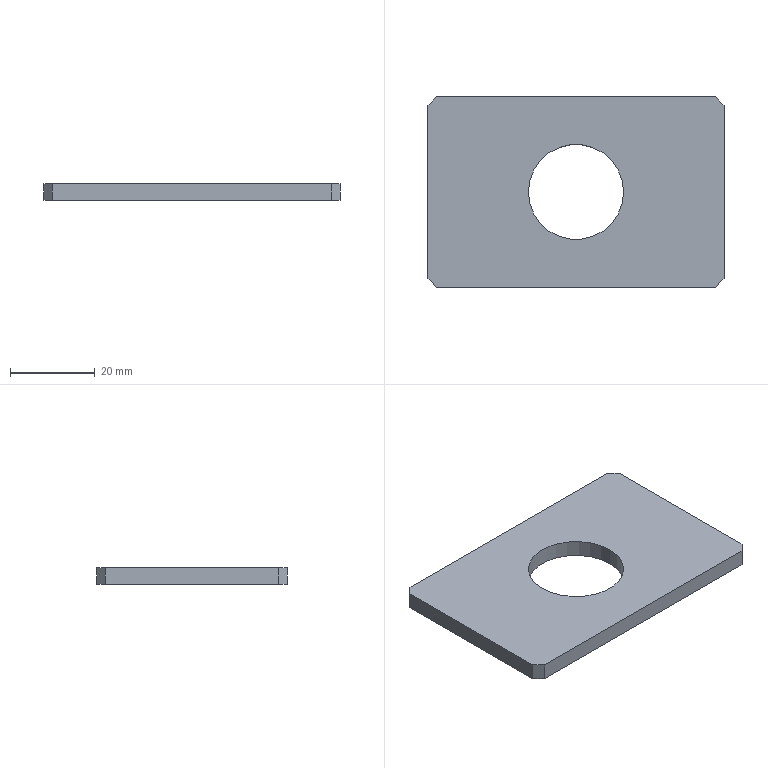Part | STEP file | Backup 2012-3-22-013 | 1 solid | 12 faces | box 70 x 45 x 4 mm | volume 10978 mm3 | plane 10 | cylinder 2 | commonest cylinder face diameters 22.5 x2
STEP:
#1=CARTESIAN_POINT('',(0.,0.,0.));
#2=DIRECTION('',(0.,0.,1.));
#3=DIRECTION('',(1.,0.,0.));
#4=AXIS2_PLACEMENT_3D('',#1,#2,#3);
#5=CARTESIAN_POINT('',(-11.25,0.,4.));
#6=VERTEX_POINT('',#5);
#7=CARTESIAN_POINT('',(-11.25,0.,0.));
#8=VERTEX_POINT('',#7);
#9=CARTESIAN_POINT('',(-11.25,0.,4.));
#10=DIRECTION('',(0.,0.,-1.));
#11=VECTOR('',#10,1.);
#12=LINE('',#9,#11);
#13=CARTESIAN_POINT('',(0.,0.,4.));
#14=DIRECTION('',(0.,0.,-1.));
#15=DIRECTION('',(-1.,0.,0.));
#16=AXIS2_PLACEMENT_3D('',#13,#14,#15);
#17=CYLINDRICAL_SURFACE('',#16,11.25);
#18=CARTESIAN_POINT('',(6.283,0.));
#19=DIRECTION('',(0.,1.));
#20=VECTOR('',#19,1.);
#21=LINE('',#18,#20);
#22=(GEOMETRIC_REPRESENTATION_CONTEXT(2)PARAMETRIC_REPRESENTATION_CONTEXT()REPRESENTATION_CONTEXT('',''));
#23=DEFINITIONAL_REPRESENTATION('',(#21),#22);
#24=PCURVE('',#17,#23);
#25=CARTESIAN_POINT('',(0.,0.,4.));
#26=DIRECTION('',(0.,0.,-1.));
#27=DIRECTION('',(-1.,0.,0.));
#28=AXIS2_PLACEMENT_3D('',#25,#26,#27);
#29=CYLINDRICAL_SURFACE('',#28,11.25);
#30=CARTESIAN_POINT('',(0.,0.));
#31=DIRECTION('',(0.,1.));
#32=VECTOR('',#31,1.);
#33=LINE('',#30,#32);
#34=(GEOMETRIC_REPRESENTATION_CONTEXT(2)PARAMETRIC_REPRESENTATION_CONTEXT()REPRESENTATION_CONTEXT('',''));
#35=DEFINITIONAL_REPRESENTATION('',(#33),#34);
#36=PCURVE('',#29,#35);
#37=SURFACE_CURVE('',#12,(#24,#36),.PCURVE_S1.);
#38=EDGE_CURVE('',#6,#8,#37,.T.);
#39=ORIENTED_EDGE('',*,*,#38,.T.);
#40=CARTESIAN_POINT('',(11.25,0.,0.));
#41=VERTEX_POINT('',#40);
#42=CARTESIAN_POINT('',(0.,0.,0.));
#43=DIRECTION('',(0.,0.,1.));
#44=DIRECTION('',(1.,0.,0.));
#45=AXIS2_PLACEMENT_3D('',#42,#43,#44);
#46=CIRCLE('',#45,11.25);
#47=CARTESIAN_POINT('',(9.425,4.));
#48=DIRECTION('',(-1.,0.));
#49=VECTOR('',#48,1.);
#50=LINE('',#47,#49);
#51=(GEOMETRIC_REPRESENTATION_CONTEXT(2)PARAMETRIC_REPRESENTATION_CONTEXT()REPRESENTATION_CONTEXT('',''));
#52=DEFINITIONAL_REPRESENTATION('',(#50),#51);
#53=PCURVE('',#17,#52);
#54=CARTESIAN_POINT('',(35.,-22.5,0.));
#55=DIRECTION('',(0.,0.,1.));
#56=DIRECTION('',(1.,0.,0.));
#57=AXIS2_PLACEMENT_3D('',#54,#55,#56);
#58=PLANE('',#57);
#59=CARTESIAN_POINT('',(-35.,22.5));
#60=DIRECTION('',(1.,0.));
#61=AXIS2_PLACEMENT_2D('',#59,#60);
#62=CIRCLE('',#61,11.25);
#63=(GEOMETRIC_REPRESENTATION_CONTEXT(2)PARAMETRIC_REPRESENTATION_CONTEXT()REPRESENTATION_CONTEXT('',''));
#64=DEFINITIONAL_REPRESENTATION('',(#62),#63);
#65=PCURVE('',#58,#64);
#66=SURFACE_CURVE('',#46,(#53,#65),.PCURVE_S1.);
#67=EDGE_CURVE('',#8,#41,#66,.T.);
#68=ORIENTED_EDGE('',*,*,#67,.T.);
#69=CARTESIAN_POINT('',(11.25,0.,4.));
#70=VERTEX_POINT('',#69);
#71=CARTESIAN_POINT('',(11.25,0.,4.));
#72=DIRECTION('',(0.,0.,-1.));
#73=VECTOR('',#72,1.);
#74=LINE('',#71,#73);
#75=CARTESIAN_POINT('',(3.142,0.));
#76=DIRECTION('',(0.,1.));
#77=VECTOR('',#76,1.);
#78=LINE('',#75,#77);
#79=(GEOMETRIC_REPRESENTATION_CONTEXT(2)PARAMETRIC_REPRESENTATION_CONTEXT()REPRESENTATION_CONTEXT('',''));
#80=DEFINITIONAL_REPRESENTATION('',(#78),#79);
#81=PCURVE('',#17,#80);
#82=CARTESIAN_POINT('',(3.142,0.));
#83=DIRECTION('',(0.,1.));
#84=VECTOR('',#83,1.);
#85=LINE('',#82,#84);
#86=(GEOMETRIC_REPRESENTATION_CONTEXT(2)PARAMETRIC_REPRESENTATION_CONTEXT()REPRESENTATION_CONTEXT('',''));
#87=DEFINITIONAL_REPRESENTATION('',(#85),#86);
#88=PCURVE('',#29,#87);
#89=SURFACE_CURVE('',#74,(#81,#88),.PCURVE_S1.);
#90=EDGE_CURVE('',#70,#41,#89,.T.);
#91=ORIENTED_EDGE('',*,*,#90,.F.);
#92=CARTESIAN_POINT('',(0.,0.,4.));
#93=DIRECTION('',(0.,0.,1.));
#94=DIRECTION('',(1.,0.,0.));
#95=AXIS2_PLACEMENT_3D('',#92,#93,#94);
#96=CIRCLE('',#95,11.25);
#97=CARTESIAN_POINT('',(9.425,0.));
#98=DIRECTION('',(-1.,0.));
#99=VECTOR('',#98,1.);
#100=LINE('',#97,#99);
#101=(GEOMETRIC_REPRESENTATION_CONTEXT(2)PARAMETRIC_REPRESENTATION_CONTEXT()REPRESENTATION_CONTEXT('',''));
#102=DEFINITIONAL_REPRESENTATION('',(#100),#101);
#103=PCURVE('',#17,#102);
#104=CARTESIAN_POINT('',(35.,-22.5,4.));
#105=DIRECTION('',(0.,0.,1.));
#106=DIRECTION('',(1.,0.,0.));
#107=AXIS2_PLACEMENT_3D('',#104,#105,#106);
#108=PLANE('',#107);
#109=CARTESIAN_POINT('',(-35.,22.5));
#110=DIRECTION('',(1.,0.));
#111=AXIS2_PLACEMENT_2D('',#109,#110);
#112=CIRCLE('',#111,11.25);
#113=(GEOMETRIC_REPRESENTATION_CONTEXT(2)PARAMETRIC_REPRESENTATION_CONTEXT()REPRESENTATION_CONTEXT('',''));
#114=DEFINITIONAL_REPRESENTATION('',(#112),#113);
#115=PCURVE('',#108,#114);
#116=SURFACE_CURVE('',#96,(#103,#115),.PCURVE_S1.);
#117=EDGE_CURVE('',#6,#70,#116,.T.);
#118=ORIENTED_EDGE('',*,*,#117,.F.);
#119=EDGE_LOOP('',(#39,#68,#91,#118));
#120=FACE_BOUND('',#119,.F.);
#121=ADVANCED_FACE('',(#120),#17,.F.);
#122=CARTESIAN_POINT('',(-35.,20.5,4.));
#123=VERTEX_POINT('',#122);
#124=CARTESIAN_POINT('',(-35.,-20.5,4.));
#125=VERTEX_POINT('',#124);
#126=CARTESIAN_POINT('',(-35.,22.5,4.));
#127=DIRECTION('',(0.,-1.,0.));
#128=VECTOR('',#127,1.);
#129=LINE('',#126,#128);
#130=CARTESIAN_POINT('',(-70.,45.));
#131=DIRECTION('',(0.,-1.));
#132=VECTOR('',#131,1.);
#133=LINE('',#130,#132);
#134=(GEOMETRIC_REPRESENTATION_CONTEXT(2)PARAMETRIC_REPRESENTATION_CONTEXT()REPRESENTATION_CONTEXT('',''));
#135=DEFINITIONAL_REPRESENTATION('',(#133),#134);
#136=PCURVE('',#108,#135);
#137=CARTESIAN_POINT('',(-35.,22.5,4.));
#138=DIRECTION('',(1.,0.,0.));
#139=DIRECTION('',(0.,1.,0.));
#140=AXIS2_PLACEMENT_3D('',#137,#138,#139);
#141=PLANE('',#140);
#142=CARTESIAN_POINT('',(0.,0.));
#143=DIRECTION('',(-1.,0.));
#144=VECTOR('',#143,1.);
#145=LINE('',#142,#144);
#146=(GEOMETRIC_REPRESENTATION_CONTEXT(2)PARAMETRIC_REPRESENTATION_CONTEXT()REPRESENTATION_CONTEXT('',''));
#147=DEFINITIONAL_REPRESENTATION('',(#145),#146);
#148=PCURVE('',#141,#147);
#149=SURFACE_CURVE('',#129,(#136,#148),.PCURVE_S1.);
#150=EDGE_CURVE('',#123,#125,#149,.T.);
#151=ORIENTED_EDGE('',*,*,#150,.T.);
#152=CARTESIAN_POINT('',(-33.,-22.5,4.));
#153=VERTEX_POINT('',#152);
#154=CARTESIAN_POINT('',(1.,-56.5,4.));
#155=DIRECTION('',(0.7071,-0.7071,0.));
#156=VECTOR('',#155,1.);
#157=LINE('',#154,#156);
#158=CARTESIAN_POINT('',(-34.,-34.));
#159=DIRECTION('',(0.7071,-0.7071));
#160=VECTOR('',#159,1.);
#161=LINE('',#158,#160);
#162=(GEOMETRIC_REPRESENTATION_CONTEXT(2)PARAMETRIC_REPRESENTATION_CONTEXT()REPRESENTATION_CONTEXT('',''));
#163=DEFINITIONAL_REPRESENTATION('',(#161),#162);
#164=PCURVE('',#108,#163);
#165=CARTESIAN_POINT('',(-33.,-22.5,4.));
#166=DIRECTION('',(0.7071,0.7071,0.));
#167=DIRECTION('',(-0.7071,0.7071,0.));
#168=AXIS2_PLACEMENT_3D('',#165,#166,#167);
#169=PLANE('',#168);
#170=CARTESIAN_POINT('',(-48.083,0.));
#171=DIRECTION('',(-1.,0.));
#172=VECTOR('',#171,1.);
#173=LINE('',#170,#172);
#174=(GEOMETRIC_REPRESENTATION_CONTEXT(2)PARAMETRIC_REPRESENTATION_CONTEXT()REPRESENTATION_CONTEXT('',''));
#175=DEFINITIONAL_REPRESENTATION('',(#173),#174);
#176=PCURVE('',#169,#175);
#177=SURFACE_CURVE('',#157,(#164,#176),.PCURVE_S1.);
#178=EDGE_CURVE('',#125,#153,#177,.T.);
#179=ORIENTED_EDGE('',*,*,#178,.T.);
#180=CARTESIAN_POINT('',(33.,-22.5,4.));
#181=VERTEX_POINT('',#180);
#182=CARTESIAN_POINT('',(-35.,-22.5,4.));
#183=DIRECTION('',(1.,0.,0.));
#184=VECTOR('',#183,1.);
#185=LINE('',#182,#184);
#186=CARTESIAN_POINT('',(-70.,0.));
#187=DIRECTION('',(1.,0.));
#188=VECTOR('',#187,1.);
#189=LINE('',#186,#188);
#190=(GEOMETRIC_REPRESENTATION_CONTEXT(2)PARAMETRIC_REPRESENTATION_CONTEXT()REPRESENTATION_CONTEXT('',''));
#191=DEFINITIONAL_REPRESENTATION('',(#189),#190);
#192=PCURVE('',#108,#191);
#193=CARTESIAN_POINT('',(-35.,-22.5,4.));
#194=DIRECTION('',(0.,1.,0.));
#195=DIRECTION('',(0.,0.,1.));
#196=AXIS2_PLACEMENT_3D('',#193,#194,#195);
#197=PLANE('',#196);
#198=CARTESIAN_POINT('',(0.,0.));
#199=DIRECTION('',(0.,1.));
#200=VECTOR('',#199,1.);
#201=LINE('',#198,#200);
#202=(GEOMETRIC_REPRESENTATION_CONTEXT(2)PARAMETRIC_REPRESENTATION_CONTEXT()REPRESENTATION_CONTEXT('',''));
#203=DEFINITIONAL_REPRESENTATION('',(#201),#202);
#204=PCURVE('',#197,#203);
#205=SURFACE_CURVE('',#185,(#192,#204),.PCURVE_S1.);
#206=EDGE_CURVE('',#153,#181,#205,.T.);
#207=ORIENTED_EDGE('',*,*,#206,.T.);
#208=CARTESIAN_POINT('',(35.,-20.5,4.));
#209=VERTEX_POINT('',#208);
#210=CARTESIAN_POINT('',(34.,-21.5,4.));
#211=DIRECTION('',(0.7071,0.7071,0.));
#212=VECTOR('',#211,1.);
#213=LINE('',#210,#212);
#214=CARTESIAN_POINT('',(-1.,1.));
#215=DIRECTION('',(0.7071,0.7071));
#216=VECTOR('',#215,1.);
#217=LINE('',#214,#216);
#218=(GEOMETRIC_REPRESENTATION_CONTEXT(2)PARAMETRIC_REPRESENTATION_CONTEXT()REPRESENTATION_CONTEXT('',''));
#219=DEFINITIONAL_REPRESENTATION('',(#217),#218);
#220=PCURVE('',#108,#219);
#221=CARTESIAN_POINT('',(35.,-20.5,4.));
#222=DIRECTION('',(-0.7071,0.7071,0.));
#223=DIRECTION('',(-0.7071,-0.7071,0.));
#224=AXIS2_PLACEMENT_3D('',#221,#222,#223);
#225=PLANE('',#224);
#226=CARTESIAN_POINT('',(1.414,0.));
#227=DIRECTION('',(-1.,0.));
#228=VECTOR('',#227,1.);
#229=LINE('',#226,#228);
#230=(GEOMETRIC_REPRESENTATION_CONTEXT(2)PARAMETRIC_REPRESENTATION_CONTEXT()REPRESENTATION_CONTEXT('',''));
#231=DEFINITIONAL_REPRESENTATION('',(#229),#230);
#232=PCURVE('',#225,#231);
#233=SURFACE_CURVE('',#213,(#220,#232),.PCURVE_S1.);
#234=EDGE_CURVE('',#181,#209,#233,.T.);
#235=ORIENTED_EDGE('',*,*,#234,.T.);
#236=CARTESIAN_POINT('',(35.,20.5,4.));
#237=VERTEX_POINT('',#236);
#238=CARTESIAN_POINT('',(35.,22.5,4.));
#239=DIRECTION('',(0.,1.,0.));
#240=VECTOR('',#239,1.);
#241=LINE('',#238,#240);
#242=CARTESIAN_POINT('',(0.,45.));
#243=DIRECTION('',(0.,1.));
#244=VECTOR('',#243,1.);
#245=LINE('',#242,#244);
#246=(GEOMETRIC_REPRESENTATION_CONTEXT(2)PARAMETRIC_REPRESENTATION_CONTEXT()REPRESENTATION_CONTEXT('',''));
#247=DEFINITIONAL_REPRESENTATION('',(#245),#246);
#248=PCURVE('',#108,#247);
#249=CARTESIAN_POINT('',(35.,22.5,4.));
#250=DIRECTION('',(-1.,0.,0.));
#251=DIRECTION('',(0.,-1.,0.));
#252=AXIS2_PLACEMENT_3D('',#249,#250,#251);
#253=PLANE('',#252);
#254=CARTESIAN_POINT('',(0.,0.));
#255=DIRECTION('',(-1.,0.));
#256=VECTOR('',#255,1.);
#257=LINE('',#254,#256);
#258=(GEOMETRIC_REPRESENTATION_CONTEXT(2)PARAMETRIC_REPRESENTATION_CONTEXT()REPRESENTATION_CONTEXT('',''));
#259=DEFINITIONAL_REPRESENTATION('',(#257),#258);
#260=PCURVE('',#253,#259);
#261=SURFACE_CURVE('',#241,(#248,#260),.PCURVE_S1.);
#262=EDGE_CURVE('',#209,#237,#261,.T.);
#263=ORIENTED_EDGE('',*,*,#262,.T.);
#264=CARTESIAN_POINT('',(33.,22.5,4.));
#265=VERTEX_POINT('',#264);
#266=CARTESIAN_POINT('',(56.5,-1.,4.));
#267=DIRECTION('',(-0.7071,0.7071,0.));
#268=VECTOR('',#267,1.);
#269=LINE('',#266,#268);
#270=CARTESIAN_POINT('',(21.5,21.5));
#271=DIRECTION('',(-0.7071,0.7071));
#272=VECTOR('',#271,1.);
#273=LINE('',#270,#272);
#274=(GEOMETRIC_REPRESENTATION_CONTEXT(2)PARAMETRIC_REPRESENTATION_CONTEXT()REPRESENTATION_CONTEXT('',''));
#275=DEFINITIONAL_REPRESENTATION('',(#273),#274);
#276=PCURVE('',#108,#275);
#277=CARTESIAN_POINT('',(33.,22.5,4.));
#278=DIRECTION('',(-0.7071,-0.7071,0.));
#279=DIRECTION('',(0.7071,-0.7071,0.));
#280=AXIS2_PLACEMENT_3D('',#277,#278,#279);
#281=PLANE('',#280);
#282=CARTESIAN_POINT('',(33.234,0.));
#283=DIRECTION('',(-1.,0.));
#284=VECTOR('',#283,1.);
#285=LINE('',#282,#284);
#286=(GEOMETRIC_REPRESENTATION_CONTEXT(2)PARAMETRIC_REPRESENTATION_CONTEXT()REPRESENTATION_CONTEXT('',''));
#287=DEFINITIONAL_REPRESENTATION('',(#285),#286);
#288=PCURVE('',#281,#287);
#289=SURFACE_CURVE('',#269,(#276,#288),.PCURVE_S1.);
#290=EDGE_CURVE('',#237,#265,#289,.T.);
#291=ORIENTED_EDGE('',*,*,#290,.T.);
#292=CARTESIAN_POINT('',(-33.,22.5,4.));
#293=VERTEX_POINT('',#292);
#294=CARTESIAN_POINT('',(-35.,22.5,4.));
#295=DIRECTION('',(-1.,0.,0.));
#296=VECTOR('',#295,1.);
#297=LINE('',#294,#296);
#298=CARTESIAN_POINT('',(-70.,45.));
#299=DIRECTION('',(-1.,0.));
#300=VECTOR('',#299,1.);
#301=LINE('',#298,#300);
#302=(GEOMETRIC_REPRESENTATION_CONTEXT(2)PARAMETRIC_REPRESENTATION_CONTEXT()REPRESENTATION_CONTEXT('',''));
#303=DEFINITIONAL_REPRESENTATION('',(#301),#302);
#304=PCURVE('',#108,#303);
#305=CARTESIAN_POINT('',(-35.,22.5,4.));
#306=DIRECTION('',(0.,-1.,0.));
#307=DIRECTION('',(0.,0.,-1.));
#308=AXIS2_PLACEMENT_3D('',#305,#306,#307);
#309=PLANE('',#308);
#310=CARTESIAN_POINT('',(0.,0.));
#311=DIRECTION('',(0.,-1.));
#312=VECTOR('',#311,1.);
#313=LINE('',#310,#312);
#314=(GEOMETRIC_REPRESENTATION_CONTEXT(2)PARAMETRIC_REPRESENTATION_CONTEXT()REPRESENTATION_CONTEXT('',''));
#315=DEFINITIONAL_REPRESENTATION('',(#313),#314);
#316=PCURVE('',#309,#315);
#317=SURFACE_CURVE('',#297,(#304,#316),.PCURVE_S1.);
#318=EDGE_CURVE('',#265,#293,#317,.T.);
#319=ORIENTED_EDGE('',*,*,#318,.T.);
#320=CARTESIAN_POINT('',(-21.5,34.,4.));
#321=DIRECTION('',(-0.7071,-0.7071,0.));
#322=VECTOR('',#321,1.);
#323=LINE('',#320,#322);
#324=CARTESIAN_POINT('',(-56.5,56.5));
#325=DIRECTION('',(-0.7071,-0.7071));
#326=VECTOR('',#325,1.);
#327=LINE('',#324,#326);
#328=(GEOMETRIC_REPRESENTATION_CONTEXT(2)PARAMETRIC_REPRESENTATION_CONTEXT()REPRESENTATION_CONTEXT('',''));
#329=DEFINITIONAL_REPRESENTATION('',(#327),#328);
#330=PCURVE('',#108,#329);
#331=CARTESIAN_POINT('',(-35.,20.5,4.));
#332=DIRECTION('',(0.7071,-0.7071,0.));
#333=DIRECTION('',(0.7071,0.7071,0.));
#334=AXIS2_PLACEMENT_3D('',#331,#332,#333);
#335=PLANE('',#334);
#336=CARTESIAN_POINT('',(19.092,0.));
#337=DIRECTION('',(-1.,0.));
#338=VECTOR('',#337,1.);
#339=LINE('',#336,#338);
#340=(GEOMETRIC_REPRESENTATION_CONTEXT(2)PARAMETRIC_REPRESENTATION_CONTEXT()REPRESENTATION_CONTEXT('',''));
#341=DEFINITIONAL_REPRESENTATION('',(#339),#340);
#342=PCURVE('',#335,#341);
#343=SURFACE_CURVE('',#323,(#330,#342),.PCURVE_S1.);
#344=EDGE_CURVE('',#293,#123,#343,.T.);
#345=ORIENTED_EDGE('',*,*,#344,.T.);
#346=EDGE_LOOP('',(#151,#179,#207,#235,#263,#291,#319,#345));
#347=FACE_BOUND('',#346,.T.);
#348=ORIENTED_EDGE('',*,*,#117,.F.);
#349=CARTESIAN_POINT('',(0.,0.,4.));
#350=DIRECTION('',(0.,0.,1.));
#351=DIRECTION('',(1.,0.,0.));
#352=AXIS2_PLACEMENT_3D('',#349,#350,#351);
#353=CIRCLE('',#352,11.25);
#354=CARTESIAN_POINT('',(-35.,22.5));
#355=DIRECTION('',(1.,0.));
#356=AXIS2_PLACEMENT_2D('',#354,#355);
#357=CIRCLE('',#356,11.25);
#358=(GEOMETRIC_REPRESENTATION_CONTEXT(2)PARAMETRIC_REPRESENTATION_CONTEXT()REPRESENTATION_CONTEXT('',''));
#359=DEFINITIONAL_REPRESENTATION('',(#357),#358);
#360=PCURVE('',#108,#359);
#361=CARTESIAN_POINT('',(3.142,0.));
#362=DIRECTION('',(-1.,0.));
#363=VECTOR('',#362,1.);
#364=LINE('',#361,#363);
#365=(GEOMETRIC_REPRESENTATION_CONTEXT(2)PARAMETRIC_REPRESENTATION_CONTEXT()REPRESENTATION_CONTEXT('',''));
#366=DEFINITIONAL_REPRESENTATION('',(#364),#365);
#367=PCURVE('',#29,#366);
#368=SURFACE_CURVE('',#353,(#360,#367),.PCURVE_S1.);
#369=EDGE_CURVE('',#70,#6,#368,.T.);
#370=ORIENTED_EDGE('',*,*,#369,.F.);
#371=EDGE_LOOP('',(#348,#370));
#372=FACE_BOUND('',#371,.T.);
#373=ADVANCED_FACE('',(#347,#372),#108,.T.);
#374=CARTESIAN_POINT('',(-33.,-22.5,0.));
#375=VERTEX_POINT('',#374);
#376=CARTESIAN_POINT('',(33.,-22.5,0.));
#377=VERTEX_POINT('',#376);
#378=CARTESIAN_POINT('',(-35.,-22.5,0.));
#379=DIRECTION('',(1.,0.,0.));
#380=VECTOR('',#379,1.);
#381=LINE('',#378,#380);
#382=CARTESIAN_POINT('',(-70.,0.));
#383=DIRECTION('',(1.,0.));
#384=VECTOR('',#383,1.);
#385=LINE('',#382,#384);
#386=(GEOMETRIC_REPRESENTATION_CONTEXT(2)PARAMETRIC_REPRESENTATION_CONTEXT()REPRESENTATION_CONTEXT('',''));
#387=DEFINITIONAL_REPRESENTATION('',(#385),#386);
#388=PCURVE('',#58,#387);
#389=CARTESIAN_POINT('',(-4.,0.));
#390=DIRECTION('',(0.,1.));
#391=VECTOR('',#390,1.);
#392=LINE('',#389,#391);
#393=(GEOMETRIC_REPRESENTATION_CONTEXT(2)PARAMETRIC_REPRESENTATION_CONTEXT()REPRESENTATION_CONTEXT('',''));
#394=DEFINITIONAL_REPRESENTATION('',(#392),#393);
#395=PCURVE('',#197,#394);
#396=SURFACE_CURVE('',#381,(#388,#395),.PCURVE_S1.);
#397=EDGE_CURVE('',#375,#377,#396,.T.);
#398=ORIENTED_EDGE('',*,*,#397,.F.);
#399=CARTESIAN_POINT('',(-35.,-20.5,0.));
#400=VERTEX_POINT('',#399);
#401=CARTESIAN_POINT('',(-33.,-22.5,0.));
#402=DIRECTION('',(-0.7071,0.7071,0.));
#403=VECTOR('',#402,1.);
#404=LINE('',#401,#403);
#405=CARTESIAN_POINT('',(-68.,0.));
#406=DIRECTION('',(-0.7071,0.7071));
#407=VECTOR('',#406,1.);
#408=LINE('',#405,#407);
#409=(GEOMETRIC_REPRESENTATION_CONTEXT(2)PARAMETRIC_REPRESENTATION_CONTEXT()REPRESENTATION_CONTEXT('',''));
#410=DEFINITIONAL_REPRESENTATION('',(#408),#409);
#411=PCURVE('',#58,#410);
#412=CARTESIAN_POINT('',(0.,-4.));
#413=DIRECTION('',(1.,0.));
#414=VECTOR('',#413,1.);
#415=LINE('',#412,#414);
#416=(GEOMETRIC_REPRESENTATION_CONTEXT(2)PARAMETRIC_REPRESENTATION_CONTEXT()REPRESENTATION_CONTEXT('',''));
#417=DEFINITIONAL_REPRESENTATION('',(#415),#416);
#418=PCURVE('',#169,#417);
#419=SURFACE_CURVE('',#404,(#411,#418),.PCURVE_S1.);
#420=EDGE_CURVE('',#375,#400,#419,.T.);
#421=ORIENTED_EDGE('',*,*,#420,.T.);
#422=CARTESIAN_POINT('',(-35.,20.5,0.));
#423=VERTEX_POINT('',#422);
#424=CARTESIAN_POINT('',(-35.,22.5,0.));
#425=DIRECTION('',(0.,-1.,0.));
#426=VECTOR('',#425,1.);
#427=LINE('',#424,#426);
#428=CARTESIAN_POINT('',(-70.,45.));
#429=DIRECTION('',(0.,-1.));
#430=VECTOR('',#429,1.);
#431=LINE('',#428,#430);
#432=(GEOMETRIC_REPRESENTATION_CONTEXT(2)PARAMETRIC_REPRESENTATION_CONTEXT()REPRESENTATION_CONTEXT('',''));
#433=DEFINITIONAL_REPRESENTATION('',(#431),#432);
#434=PCURVE('',#58,#433);
#435=CARTESIAN_POINT('',(0.,-4.));
#436=DIRECTION('',(-1.,0.));
#437=VECTOR('',#436,1.);
#438=LINE('',#435,#437);
#439=(GEOMETRIC_REPRESENTATION_CONTEXT(2)PARAMETRIC_REPRESENTATION_CONTEXT()REPRESENTATION_CONTEXT('',''));
#440=DEFINITIONAL_REPRESENTATION('',(#438),#439);
#441=PCURVE('',#141,#440);
#442=SURFACE_CURVE('',#427,(#434,#441),.PCURVE_S1.);
#443=EDGE_CURVE('',#423,#400,#442,.T.);
#444=ORIENTED_EDGE('',*,*,#443,.F.);
#445=CARTESIAN_POINT('',(-33.,22.5,0.));
#446=VERTEX_POINT('',#445);
#447=CARTESIAN_POINT('',(-35.,20.5,0.));
#448=DIRECTION('',(0.7071,0.7071,0.));
#449=VECTOR('',#448,1.);
#450=LINE('',#447,#449);
#451=CARTESIAN_POINT('',(-70.,43.));
#452=DIRECTION('',(0.7071,0.7071));
#453=VECTOR('',#452,1.);
#454=LINE('',#451,#453);
#455=(GEOMETRIC_REPRESENTATION_CONTEXT(2)PARAMETRIC_REPRESENTATION_CONTEXT()REPRESENTATION_CONTEXT('',''));
#456=DEFINITIONAL_REPRESENTATION('',(#454),#455);
#457=PCURVE('',#58,#456);
#458=CARTESIAN_POINT('',(0.,-4.));
#459=DIRECTION('',(1.,0.));
#460=VECTOR('',#459,1.);
#461=LINE('',#458,#460);
#462=(GEOMETRIC_REPRESENTATION_CONTEXT(2)PARAMETRIC_REPRESENTATION_CONTEXT()REPRESENTATION_CONTEXT('',''));
#463=DEFINITIONAL_REPRESENTATION('',(#461),#462);
#464=PCURVE('',#335,#463);
#465=SURFACE_CURVE('',#450,(#457,#464),.PCURVE_S1.);
#466=EDGE_CURVE('',#423,#446,#465,.T.);
#467=ORIENTED_EDGE('',*,*,#466,.T.);
#468=CARTESIAN_POINT('',(33.,22.5,0.));
#469=VERTEX_POINT('',#468);
#470=CARTESIAN_POINT('',(-35.,22.5,0.));
#471=DIRECTION('',(-1.,0.,0.));
#472=VECTOR('',#471,1.);
#473=LINE('',#470,#472);
#474=CARTESIAN_POINT('',(-70.,45.));
#475=DIRECTION('',(-1.,0.));
#476=VECTOR('',#475,1.);
#477=LINE('',#474,#476);
#478=(GEOMETRIC_REPRESENTATION_CONTEXT(2)PARAMETRIC_REPRESENTATION_CONTEXT()REPRESENTATION_CONTEXT('',''));
#479=DEFINITIONAL_REPRESENTATION('',(#477),#478);
#480=PCURVE('',#58,#479);
#481=CARTESIAN_POINT('',(4.,0.));
#482=DIRECTION('',(0.,-1.));
#483=VECTOR('',#482,1.);
#484=LINE('',#481,#483);
#485=(GEOMETRIC_REPRESENTATION_CONTEXT(2)PARAMETRIC_REPRESENTATION_CONTEXT()REPRESENTATION_CONTEXT('',''));
#486=DEFINITIONAL_REPRESENTATION('',(#484),#485);
#487=PCURVE('',#309,#486);
#488=SURFACE_CURVE('',#473,(#480,#487),.PCURVE_S1.);
#489=EDGE_CURVE('',#469,#446,#488,.T.);
#490=ORIENTED_EDGE('',*,*,#489,.F.);
#491=CARTESIAN_POINT('',(35.,20.5,0.));
#492=VERTEX_POINT('',#491);
#493=CARTESIAN_POINT('',(33.,22.5,0.));
#494=DIRECTION('',(0.7071,-0.7071,0.));
#495=VECTOR('',#494,1.);
#496=LINE('',#493,#495);
#497=CARTESIAN_POINT('',(-2.,45.));
#498=DIRECTION('',(0.7071,-0.7071));
#499=VECTOR('',#498,1.);
#500=LINE('',#497,#499);
#501=(GEOMETRIC_REPRESENTATION_CONTEXT(2)PARAMETRIC_REPRESENTATION_CONTEXT()REPRESENTATION_CONTEXT('',''));
#502=DEFINITIONAL_REPRESENTATION('',(#500),#501);
#503=PCURVE('',#58,#502);
#504=CARTESIAN_POINT('',(0.,-4.));
#505=DIRECTION('',(1.,0.));
#506=VECTOR('',#505,1.);
#507=LINE('',#504,#506);
#508=(GEOMETRIC_REPRESENTATION_CONTEXT(2)PARAMETRIC_REPRESENTATION_CONTEXT()REPRESENTATION_CONTEXT('',''));
#509=DEFINITIONAL_REPRESENTATION('',(#507),#508);
#510=PCURVE('',#281,#509);
#511=SURFACE_CURVE('',#496,(#503,#510),.PCURVE_S1.);
#512=EDGE_CURVE('',#469,#492,#511,.T.);
#513=ORIENTED_EDGE('',*,*,#512,.T.);
#514=CARTESIAN_POINT('',(35.,-20.5,0.));
#515=VERTEX_POINT('',#514);
#516=CARTESIAN_POINT('',(35.,22.5,0.));
#517=DIRECTION('',(0.,1.,0.));
#518=VECTOR('',#517,1.);
#519=LINE('',#516,#518);
#520=CARTESIAN_POINT('',(0.,45.));
#521=DIRECTION('',(0.,1.));
#522=VECTOR('',#521,1.);
#523=LINE('',#520,#522);
#524=(GEOMETRIC_REPRESENTATION_CONTEXT(2)PARAMETRIC_REPRESENTATION_CONTEXT()REPRESENTATION_CONTEXT('',''));
#525=DEFINITIONAL_REPRESENTATION('',(#523),#524);
#526=PCURVE('',#58,#525);
#527=CARTESIAN_POINT('',(0.,-4.));
#528=DIRECTION('',(-1.,0.));
#529=VECTOR('',#528,1.);
#530=LINE('',#527,#529);
#531=(GEOMETRIC_REPRESENTATION_CONTEXT(2)PARAMETRIC_REPRESENTATION_CONTEXT()REPRESENTATION_CONTEXT('',''));
#532=DEFINITIONAL_REPRESENTATION('',(#530),#531);
#533=PCURVE('',#253,#532);
#534=SURFACE_CURVE('',#519,(#526,#533),.PCURVE_S1.);
#535=EDGE_CURVE('',#515,#492,#534,.T.);
#536=ORIENTED_EDGE('',*,*,#535,.F.);
#537=CARTESIAN_POINT('',(35.,-20.5,0.));
#538=DIRECTION('',(-0.7071,-0.7071,0.));
#539=VECTOR('',#538,1.);
#540=LINE('',#537,#539);
#541=CARTESIAN_POINT('',(0.,2.));
#542=DIRECTION('',(-0.7071,-0.7071));
#543=VECTOR('',#542,1.);
#544=LINE('',#541,#543);
#545=(GEOMETRIC_REPRESENTATION_CONTEXT(2)PARAMETRIC_REPRESENTATION_CONTEXT()REPRESENTATION_CONTEXT('',''));
#546=DEFINITIONAL_REPRESENTATION('',(#544),#545);
#547=PCURVE('',#58,#546);
#548=CARTESIAN_POINT('',(0.,-4.));
#549=DIRECTION('',(1.,0.));
#550=VECTOR('',#549,1.);
#551=LINE('',#548,#550);
#552=(GEOMETRIC_REPRESENTATION_CONTEXT(2)PARAMETRIC_REPRESENTATION_CONTEXT()REPRESENTATION_CONTEXT('',''));
#553=DEFINITIONAL_REPRESENTATION('',(#551),#552);
#554=PCURVE('',#225,#553);
#555=SURFACE_CURVE('',#540,(#547,#554),.PCURVE_S1.);
#556=EDGE_CURVE('',#515,#377,#555,.T.);
#557=ORIENTED_EDGE('',*,*,#556,.T.);
#558=EDGE_LOOP('',(#398,#421,#444,#467,#490,#513,#536,#557));
#559=FACE_BOUND('',#558,.T.);
#560=ORIENTED_EDGE('',*,*,#67,.T.);
#561=CARTESIAN_POINT('',(0.,0.,0.));
#562=DIRECTION('',(0.,0.,1.));
#563=DIRECTION('',(1.,0.,0.));
#564=AXIS2_PLACEMENT_3D('',#561,#562,#563);
#565=CIRCLE('',#564,11.25);
#566=CARTESIAN_POINT('',(-35.,22.5));
#567=DIRECTION('',(1.,0.));
#568=AXIS2_PLACEMENT_2D('',#566,#567);
#569=CIRCLE('',#568,11.25);
#570=(GEOMETRIC_REPRESENTATION_CONTEXT(2)PARAMETRIC_REPRESENTATION_CONTEXT()REPRESENTATION_CONTEXT('',''));
#571=DEFINITIONAL_REPRESENTATION('',(#569),#570);
#572=PCURVE('',#58,#571);
#573=CARTESIAN_POINT('',(3.142,4.));
#574=DIRECTION('',(-1.,0.));
#575=VECTOR('',#574,1.);
#576=LINE('',#573,#575);
#577=(GEOMETRIC_REPRESENTATION_CONTEXT(2)PARAMETRIC_REPRESENTATION_CONTEXT()REPRESENTATION_CONTEXT('',''));
#578=DEFINITIONAL_REPRESENTATION('',(#576),#577);
#579=PCURVE('',#29,#578);
#580=SURFACE_CURVE('',#565,(#572,#579),.PCURVE_S1.);
#581=EDGE_CURVE('',#41,#8,#580,.T.);
#582=ORIENTED_EDGE('',*,*,#581,.T.);
#583=EDGE_LOOP('',(#560,#582));
#584=FACE_BOUND('',#583,.T.);
#585=ADVANCED_FACE('',(#559,#584),#58,.F.);
#586=ORIENTED_EDGE('',*,*,#262,.F.);
#587=CARTESIAN_POINT('',(35.,-20.5,4.));
#588=DIRECTION('',(0.,0.,-1.));
#589=VECTOR('',#588,1.);
#590=LINE('',#587,#589);
#591=CARTESIAN_POINT('',(43.,0.));
#592=DIRECTION('',(0.,-1.));
#593=VECTOR('',#592,1.);
#594=LINE('',#591,#593);
#595=(GEOMETRIC_REPRESENTATION_CONTEXT(2)PARAMETRIC_REPRESENTATION_CONTEXT()REPRESENTATION_CONTEXT('',''));
#596=DEFINITIONAL_REPRESENTATION('',(#594),#595);
#597=PCURVE('',#253,#596);
#598=CARTESIAN_POINT('',(0.,0.));
#599=DIRECTION('',(0.,-1.));
#600=VECTOR('',#599,1.);
#601=LINE('',#598,#600);
#602=(GEOMETRIC_REPRESENTATION_CONTEXT(2)PARAMETRIC_REPRESENTATION_CONTEXT()REPRESENTATION_CONTEXT('',''));
#603=DEFINITIONAL_REPRESENTATION('',(#601),#602);
#604=PCURVE('',#225,#603);
#605=SURFACE_CURVE('',#590,(#597,#604),.PCURVE_S1.);
#606=EDGE_CURVE('',#209,#515,#605,.T.);
#607=ORIENTED_EDGE('',*,*,#606,.T.);
#608=ORIENTED_EDGE('',*,*,#535,.T.);
#609=CARTESIAN_POINT('',(35.,20.5,4.));
#610=DIRECTION('',(0.,0.,1.));
#611=VECTOR('',#610,1.);
#612=LINE('',#609,#611);
#613=CARTESIAN_POINT('',(2.,0.));
#614=DIRECTION('',(0.,1.));
#615=VECTOR('',#614,1.);
#616=LINE('',#613,#615);
#617=(GEOMETRIC_REPRESENTATION_CONTEXT(2)PARAMETRIC_REPRESENTATION_CONTEXT()REPRESENTATION_CONTEXT('',''));
#618=DEFINITIONAL_REPRESENTATION('',(#616),#617);
#619=PCURVE('',#253,#618);
#620=CARTESIAN_POINT('',(2.828,0.));
#621=DIRECTION('',(0.,1.));
#622=VECTOR('',#621,1.);
#623=LINE('',#620,#622);
#624=(GEOMETRIC_REPRESENTATION_CONTEXT(2)PARAMETRIC_REPRESENTATION_CONTEXT()REPRESENTATION_CONTEXT('',''));
#625=DEFINITIONAL_REPRESENTATION('',(#623),#624);
#626=PCURVE('',#281,#625);
#627=SURFACE_CURVE('',#612,(#619,#626),.PCURVE_S1.);
#628=EDGE_CURVE('',#492,#237,#627,.T.);
#629=ORIENTED_EDGE('',*,*,#628,.T.);
#630=EDGE_LOOP('',(#586,#607,#608,#629));
#631=FACE_BOUND('',#630,.T.);
#632=ADVANCED_FACE('',(#631),#253,.F.);
#633=ORIENTED_EDGE('',*,*,#489,.T.);
#634=CARTESIAN_POINT('',(-33.,22.5,4.));
#635=DIRECTION('',(0.,0.,1.));
#636=VECTOR('',#635,1.);
#637=LINE('',#634,#636);
#638=CARTESIAN_POINT('',(0.,2.));
#639=DIRECTION('',(-1.,0.));
#640=VECTOR('',#639,1.);
#641=LINE('',#638,#640);
#642=(GEOMETRIC_REPRESENTATION_CONTEXT(2)PARAMETRIC_REPRESENTATION_CONTEXT()REPRESENTATION_CONTEXT('',''));
#643=DEFINITIONAL_REPRESENTATION('',(#641),#642);
#644=PCURVE('',#309,#643);
#645=CARTESIAN_POINT('',(2.828,0.));
#646=DIRECTION('',(0.,1.));
#647=VECTOR('',#646,1.);
#648=LINE('',#645,#647);
#649=(GEOMETRIC_REPRESENTATION_CONTEXT(2)PARAMETRIC_REPRESENTATION_CONTEXT()REPRESENTATION_CONTEXT('',''));
#650=DEFINITIONAL_REPRESENTATION('',(#648),#649);
#651=PCURVE('',#335,#650);
#652=SURFACE_CURVE('',#637,(#644,#651),.PCURVE_S1.);
#653=EDGE_CURVE('',#446,#293,#652,.T.);
#654=ORIENTED_EDGE('',*,*,#653,.T.);
#655=ORIENTED_EDGE('',*,*,#318,.F.);
#656=CARTESIAN_POINT('',(33.,22.5,4.));
#657=DIRECTION('',(0.,0.,-1.));
#658=VECTOR('',#657,1.);
#659=LINE('',#656,#658);
#660=CARTESIAN_POINT('',(0.,68.));
#661=DIRECTION('',(1.,0.));
#662=VECTOR('',#661,1.);
#663=LINE('',#660,#662);
#664=(GEOMETRIC_REPRESENTATION_CONTEXT(2)PARAMETRIC_REPRESENTATION_CONTEXT()REPRESENTATION_CONTEXT('',''));
#665=DEFINITIONAL_REPRESENTATION('',(#663),#664);
#666=PCURVE('',#309,#665);
#667=CARTESIAN_POINT('',(0.,0.));
#668=DIRECTION('',(0.,-1.));
#669=VECTOR('',#668,1.);
#670=LINE('',#667,#669);
#671=(GEOMETRIC_REPRESENTATION_CONTEXT(2)PARAMETRIC_REPRESENTATION_CONTEXT()REPRESENTATION_CONTEXT('',''));
#672=DEFINITIONAL_REPRESENTATION('',(#670),#671);
#673=PCURVE('',#281,#672);
#674=SURFACE_CURVE('',#659,(#666,#673),.PCURVE_S1.);
#675=EDGE_CURVE('',#265,#469,#674,.T.);
#676=ORIENTED_EDGE('',*,*,#675,.T.);
#677=EDGE_LOOP('',(#633,#654,#655,#676));
#678=FACE_BOUND('',#677,.T.);
#679=ADVANCED_FACE('',(#678),#309,.F.);
#680=ORIENTED_EDGE('',*,*,#443,.T.);
#681=CARTESIAN_POINT('',(-35.,-20.5,4.));
#682=DIRECTION('',(0.,0.,1.));
#683=VECTOR('',#682,1.);
#684=LINE('',#681,#683);
#685=CARTESIAN_POINT('',(-43.,0.));
#686=DIRECTION('',(0.,1.));
#687=VECTOR('',#686,1.);
#688=LINE('',#685,#687);
#689=(GEOMETRIC_REPRESENTATION_CONTEXT(2)PARAMETRIC_REPRESENTATION_CONTEXT()REPRESENTATION_CONTEXT('',''));
#690=DEFINITIONAL_REPRESENTATION('',(#688),#689);
#691=PCURVE('',#141,#690);
#692=CARTESIAN_POINT('',(2.828,0.));
#693=DIRECTION('',(0.,1.));
#694=VECTOR('',#693,1.);
#695=LINE('',#692,#694);
#696=(GEOMETRIC_REPRESENTATION_CONTEXT(2)PARAMETRIC_REPRESENTATION_CONTEXT()REPRESENTATION_CONTEXT('',''));
#697=DEFINITIONAL_REPRESENTATION('',(#695),#696);
#698=PCURVE('',#169,#697);
#699=SURFACE_CURVE('',#684,(#691,#698),.PCURVE_S1.);
#700=EDGE_CURVE('',#400,#125,#699,.T.);
#701=ORIENTED_EDGE('',*,*,#700,.T.);
#702=ORIENTED_EDGE('',*,*,#150,.F.);
#703=CARTESIAN_POINT('',(-35.,20.5,4.));
#704=DIRECTION('',(0.,0.,-1.));
#705=VECTOR('',#704,1.);
#706=LINE('',#703,#705);
#707=CARTESIAN_POINT('',(-2.,0.));
#708=DIRECTION('',(0.,-1.));
#709=VECTOR('',#708,1.);
#710=LINE('',#707,#709);
#711=(GEOMETRIC_REPRESENTATION_CONTEXT(2)PARAMETRIC_REPRESENTATION_CONTEXT()REPRESENTATION_CONTEXT('',''));
#712=DEFINITIONAL_REPRESENTATION('',(#710),#711);
#713=PCURVE('',#141,#712);
#714=CARTESIAN_POINT('',(0.,0.));
#715=DIRECTION('',(0.,-1.));
#716=VECTOR('',#715,1.);
#717=LINE('',#714,#716);
#718=(GEOMETRIC_REPRESENTATION_CONTEXT(2)PARAMETRIC_REPRESENTATION_CONTEXT()REPRESENTATION_CONTEXT('',''));
#719=DEFINITIONAL_REPRESENTATION('',(#717),#718);
#720=PCURVE('',#335,#719);
#721=SURFACE_CURVE('',#706,(#713,#720),.PCURVE_S1.);
#722=EDGE_CURVE('',#123,#423,#721,.T.);
#723=ORIENTED_EDGE('',*,*,#722,.T.);
#724=EDGE_LOOP('',(#680,#701,#702,#723));
#725=FACE_BOUND('',#724,.T.);
#726=ADVANCED_FACE('',(#725),#141,.F.);
#727=ORIENTED_EDGE('',*,*,#206,.F.);
#728=CARTESIAN_POINT('',(-33.,-22.5,4.));
#729=DIRECTION('',(0.,0.,-1.));
#730=VECTOR('',#729,1.);
#731=LINE('',#728,#730);
#732=CARTESIAN_POINT('',(0.,2.));
#733=DIRECTION('',(-1.,0.));
#734=VECTOR('',#733,1.);
#735=LINE('',#732,#734);
#736=(GEOMETRIC_REPRESENTATION_CONTEXT(2)PARAMETRIC_REPRESENTATION_CONTEXT()REPRESENTATION_CONTEXT('',''));
#737=DEFINITIONAL_REPRESENTATION('',(#735),#736);
#738=PCURVE('',#197,#737);
#739=CARTESIAN_POINT('',(0.,0.));
#740=DIRECTION('',(0.,-1.));
#741=VECTOR('',#740,1.);
#742=LINE('',#739,#741);
#743=(GEOMETRIC_REPRESENTATION_CONTEXT(2)PARAMETRIC_REPRESENTATION_CONTEXT()REPRESENTATION_CONTEXT('',''));
#744=DEFINITIONAL_REPRESENTATION('',(#742),#743);
#745=PCURVE('',#169,#744);
#746=SURFACE_CURVE('',#731,(#738,#745),.PCURVE_S1.);
#747=EDGE_CURVE('',#153,#375,#746,.T.);
#748=ORIENTED_EDGE('',*,*,#747,.T.);
#749=ORIENTED_EDGE('',*,*,#397,.T.);
#750=CARTESIAN_POINT('',(33.,-22.5,4.));
#751=DIRECTION('',(0.,0.,1.));
#752=VECTOR('',#751,1.);
#753=LINE('',#750,#752);
#754=CARTESIAN_POINT('',(0.,68.));
#755=DIRECTION('',(1.,0.));
#756=VECTOR('',#755,1.);
#757=LINE('',#754,#756);
#758=(GEOMETRIC_REPRESENTATION_CONTEXT(2)PARAMETRIC_REPRESENTATION_CONTEXT()REPRESENTATION_CONTEXT('',''));
#759=DEFINITIONAL_REPRESENTATION('',(#757),#758);
#760=PCURVE('',#197,#759);
#761=CARTESIAN_POINT('',(2.828,0.));
#762=DIRECTION('',(0.,1.));
#763=VECTOR('',#762,1.);
#764=LINE('',#761,#763);
#765=(GEOMETRIC_REPRESENTATION_CONTEXT(2)PARAMETRIC_REPRESENTATION_CONTEXT()REPRESENTATION_CONTEXT('',''));
#766=DEFINITIONAL_REPRESENTATION('',(#764),#765);
#767=PCURVE('',#225,#766);
#768=SURFACE_CURVE('',#753,(#760,#767),.PCURVE_S1.);
#769=EDGE_CURVE('',#377,#181,#768,.T.);
#770=ORIENTED_EDGE('',*,*,#769,.T.);
#771=EDGE_LOOP('',(#727,#748,#749,#770));
#772=FACE_BOUND('',#771,.T.);
#773=ADVANCED_FACE('',(#772),#197,.F.);
#774=ORIENTED_EDGE('',*,*,#581,.T.);
#775=ORIENTED_EDGE('',*,*,#38,.F.);
#776=ORIENTED_EDGE('',*,*,#369,.F.);
#777=ORIENTED_EDGE('',*,*,#90,.T.);
#778=EDGE_LOOP('',(#774,#775,#776,#777));
#779=FACE_BOUND('',#778,.F.);
#780=ADVANCED_FACE('',(#779),#29,.F.);
#781=ORIENTED_EDGE('',*,*,#178,.F.);
#782=ORIENTED_EDGE('',*,*,#700,.F.);
#783=ORIENTED_EDGE('',*,*,#420,.F.);
#784=ORIENTED_EDGE('',*,*,#747,.F.);
#785=EDGE_LOOP('',(#781,#782,#783,#784));
#786=FACE_BOUND('',#785,.T.);
#787=ADVANCED_FACE('',(#786),#169,.F.);
#788=ORIENTED_EDGE('',*,*,#344,.F.);
#789=ORIENTED_EDGE('',*,*,#653,.F.);
#790=ORIENTED_EDGE('',*,*,#466,.F.);
#791=ORIENTED_EDGE('',*,*,#722,.F.);
#792=EDGE_LOOP('',(#788,#789,#790,#791));
#793=FACE_BOUND('',#792,.T.);
#794=ADVANCED_FACE('',(#793),#335,.F.);
#795=ORIENTED_EDGE('',*,*,#234,.F.);
#796=ORIENTED_EDGE('',*,*,#769,.F.);
#797=ORIENTED_EDGE('',*,*,#556,.F.);
#798=ORIENTED_EDGE('',*,*,#606,.F.);
#799=EDGE_LOOP('',(#795,#796,#797,#798));
#800=FACE_BOUND('',#799,.T.);
#801=ADVANCED_FACE('',(#800),#225,.F.);
#802=ORIENTED_EDGE('',*,*,#290,.F.);
#803=ORIENTED_EDGE('',*,*,#628,.F.);
#804=ORIENTED_EDGE('',*,*,#512,.F.);
#805=ORIENTED_EDGE('',*,*,#675,.F.);
#806=EDGE_LOOP('',(#802,#803,#804,#805));
#807=FACE_BOUND('',#806,.T.);
#808=ADVANCED_FACE('',(#807),#281,.F.);
#809=CLOSED_SHELL('',(#121,#373,#585,#632,#679,#726,#773,#780,#787,#794,#801,#808));
#810=MANIFOLD_SOLID_BREP('',#809);
#811=(LENGTH_UNIT()NAMED_UNIT(*)SI_UNIT(.MILLI.,.METRE.));
#812=UNCERTAINTY_MEASURE_WITH_UNIT(LENGTH_MEASURE(0.0000001),#811,'','');
#813=(NAMED_UNIT(*)PLANE_ANGLE_UNIT()SI_UNIT($,.RADIAN.));
#814=(NAMED_UNIT(*)SI_UNIT($,.STERADIAN.)SOLID_ANGLE_UNIT());
#815=(GEOMETRIC_REPRESENTATION_CONTEXT(3)GLOBAL_UNCERTAINTY_ASSIGNED_CONTEXT((#812))GLOBAL_UNIT_ASSIGNED_CONTEXT((#811,#813,#814))REPRESENTATION_CONTEXT('',''));
#816=ADVANCED_BREP_SHAPE_REPRESENTATION('',(#4,#810),#815);